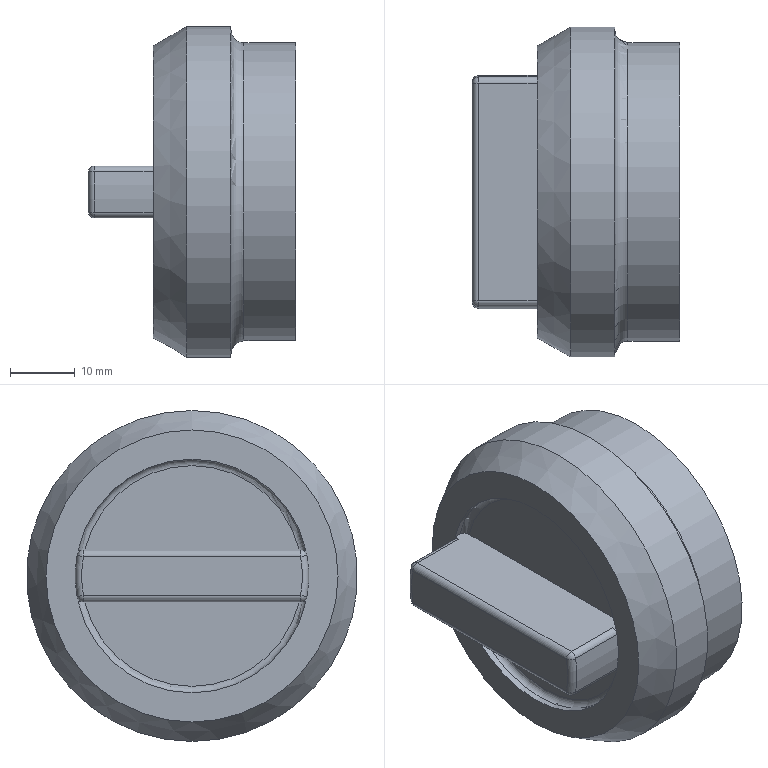Part | NX | features BLEND 3, DATUM_CSYS 3, SKETCH 2, CHAMFER 1, CYLINDER 1, EXTRUDE 1, HOLE PACKAGE 1, SIMPLE HOLE 1, SWP104 1, SYMBOLIC_THREAD 1 | 1 solid | 36 faces | box 32 x 51 x 51 mm | volume 28582 mm3 | cylinder 14 | plane 10 | torus 5 | sphere 4 | cone 3 | commonest cylinder face diameters 2 x6 36 x4 33 x1 36.5 x1 46 x1 51 x1
STEP:
#1=CARTESIAN_POINT('',(-21.,-17.55,4.));
#2=VERTEX_POINT('',#1);
#3=CARTESIAN_POINT('',(-22.,-17.55,4.));
#4=VERTEX_POINT('',#3);
#5=CARTESIAN_POINT('',(-32.,-17.55,4.));
#6=DIRECTION('',(1.,0.,0.));
#7=VECTOR('',#6,1000.);
#8=LINE('',#5,#7);
#9=EDGE_CURVE('',#2,#4,#8,.F.);
#10=ORIENTED_EDGE('',*,*,#9,.T.);
#11=CARTESIAN_POINT('',(-22.,17.55,4.));
#12=VERTEX_POINT('',#11);
#13=CARTESIAN_POINT('',(-22.,0.,0.));
#14=DIRECTION('',(-1.,0.,0.));
#15=DIRECTION('',(0.,0.,1.));
#16=AXIS2_PLACEMENT_3D('',#13,#14,#15);
#17=CIRCLE('',#16,18.);
#18=EDGE_CURVE('',#4,#12,#17,.T.);
#19=ORIENTED_EDGE('',*,*,#18,.T.);
#20=CARTESIAN_POINT('',(-21.,17.55,4.));
#21=VERTEX_POINT('',#20);
#22=CARTESIAN_POINT('',(-32.,17.55,4.));
#23=DIRECTION('',(1.,0.,0.));
#24=VECTOR('',#23,1000.);
#25=LINE('',#22,#24);
#26=EDGE_CURVE('',#12,#21,#25,.T.);
#27=ORIENTED_EDGE('',*,*,#26,.T.);
#28=CARTESIAN_POINT('',(-21.,0.,0.));
#29=DIRECTION('',(-1.,0.,0.));
#30=DIRECTION('',(0.,0.,1.));
#31=AXIS2_PLACEMENT_3D('',#28,#29,#30);
#32=CIRCLE('',#31,18.);
#33=EDGE_CURVE('',#2,#21,#32,.T.);
#34=ORIENTED_EDGE('',*,*,#33,.F.);
#35=EDGE_LOOP('',(#10,#19,#27,#34));
#36=FACE_BOUND('',#35,.T.);
#37=CARTESIAN_POINT('',(0.,0.,0.));
#38=DIRECTION('',(-1.,0.,0.));
#39=DIRECTION('',(0.,0.,1.));
#40=AXIS2_PLACEMENT_3D('',#37,#38,#39);
#41=CYLINDRICAL_SURFACE('',#40,18.);
#42=ADVANCED_FACE('',(#36),#41,.F.);
#43=CARTESIAN_POINT('',(-22.,17.55,-4.));
#44=VERTEX_POINT('',#43);
#45=CARTESIAN_POINT('',(-22.,-17.55,-4.));
#46=VERTEX_POINT('',#45);
#47=CARTESIAN_POINT('',(-22.,0.,0.));
#48=DIRECTION('',(-1.,0.,0.));
#49=DIRECTION('',(0.,0.,1.));
#50=AXIS2_PLACEMENT_3D('',#47,#48,#49);
#51=CIRCLE('',#50,18.);
#52=EDGE_CURVE('',#44,#46,#51,.T.);
#53=ORIENTED_EDGE('',*,*,#52,.T.);
#54=CARTESIAN_POINT('',(-21.,-17.55,-4.));
#55=VERTEX_POINT('',#54);
#56=CARTESIAN_POINT('',(-32.,-17.55,-4.));
#57=DIRECTION('',(1.,0.,0.));
#58=VECTOR('',#57,1000.);
#59=LINE('',#56,#58);
#60=EDGE_CURVE('',#46,#55,#59,.T.);
#61=ORIENTED_EDGE('',*,*,#60,.T.);
#62=CARTESIAN_POINT('',(-21.,17.55,-4.));
#63=VERTEX_POINT('',#62);
#64=CARTESIAN_POINT('',(-21.,0.,0.));
#65=DIRECTION('',(-1.,0.,0.));
#66=DIRECTION('',(0.,0.,1.));
#67=AXIS2_PLACEMENT_3D('',#64,#65,#66);
#68=CIRCLE('',#67,18.);
#69=EDGE_CURVE('',#63,#55,#68,.T.);
#70=ORIENTED_EDGE('',*,*,#69,.F.);
#71=CARTESIAN_POINT('',(-32.,17.55,-4.));
#72=DIRECTION('',(1.,0.,0.));
#73=VECTOR('',#72,1000.);
#74=LINE('',#71,#73);
#75=EDGE_CURVE('',#63,#44,#74,.F.);
#76=ORIENTED_EDGE('',*,*,#75,.T.);
#77=EDGE_LOOP('',(#53,#61,#70,#76));
#78=FACE_BOUND('',#77,.T.);
#79=CARTESIAN_POINT('',(0.,0.,0.));
#80=DIRECTION('',(-1.,0.,0.));
#81=DIRECTION('',(0.,0.,1.));
#82=AXIS2_PLACEMENT_3D('',#79,#80,#81);
#83=CYLINDRICAL_SURFACE('',#82,18.);
#84=ADVANCED_FACE('',(#78),#83,.F.);
#85=CARTESIAN_POINT('',(-20.,-16.523,4.));
#86=VERTEX_POINT('',#85);
#87=CARTESIAN_POINT('',(-21.,-17.55,4.));
#88=CARTESIAN_POINT('',(-20.472,-17.55,4.));
#89=CARTESIAN_POINT('',(-20.,-17.052,4.));
#90=CARTESIAN_POINT('',(-20.,-16.523,4.));
#91=B_SPLINE_CURVE_WITH_KNOTS('',3,(#87,#88,#89,#90),.UNSPECIFIED.,.F.,.F.,(4,4),(0.006013,0.007597),.UNSPECIFIED.);
#92=EDGE_CURVE('',#2,#86,#91,.T.);
#93=ORIENTED_EDGE('',*,*,#92,.F.);
#94=ORIENTED_EDGE('',*,*,#33,.T.);
#95=CARTESIAN_POINT('',(-20.,16.523,4.));
#96=VERTEX_POINT('',#95);
#97=CARTESIAN_POINT('',(-20.,16.523,4.));
#98=CARTESIAN_POINT('',(-20.,17.055,4.));
#99=CARTESIAN_POINT('',(-20.471,17.55,4.));
#100=CARTESIAN_POINT('',(-21.,17.55,4.));
#101=B_SPLINE_CURVE_WITH_KNOTS('',3,(#97,#98,#99,#100),.UNSPECIFIED.,.F.,.F.,(4,4),(0.001306,0.002891),.UNSPECIFIED.);
#102=EDGE_CURVE('',#96,#21,#101,.T.);
#103=ORIENTED_EDGE('',*,*,#102,.F.);
#104=CARTESIAN_POINT('',(-20.,0.,0.));
#105=DIRECTION('',(-1.,0.,0.));
#106=DIRECTION('',(0.,0.,1.));
#107=AXIS2_PLACEMENT_3D('',#104,#105,#106);
#108=CIRCLE('',#107,17.);
#109=EDGE_CURVE('',#86,#96,#108,.T.);
#110=ORIENTED_EDGE('',*,*,#109,.F.);
#111=EDGE_LOOP('',(#93,#94,#103,#110));
#112=FACE_BOUND('',#111,.T.);
#113=CARTESIAN_POINT('',(-21.,0.,0.));
#114=DIRECTION('',(-1.,0.,0.));
#115=DIRECTION('',(0.,0.,1.));
#116=AXIS2_PLACEMENT_3D('',#113,#114,#115);
#117=TOROIDAL_SURFACE('',#116,17.,1.);
#118=ADVANCED_FACE('',(#112),#117,.F.);
#119=CARTESIAN_POINT('',(-20.,-16.523,-4.));
#120=VERTEX_POINT('',#119);
#121=CARTESIAN_POINT('',(-20.,-16.523,-4.));
#122=CARTESIAN_POINT('',(-20.,-17.057,-4.));
#123=CARTESIAN_POINT('',(-20.464,-17.55,-4.));
#124=CARTESIAN_POINT('',(-21.,-17.55,-4.));
#125=B_SPLINE_CURVE_WITH_KNOTS('',3,(#121,#122,#123,#124),.UNSPECIFIED.,.F.,.F.,(4,4),(0.005091,0.006676),.UNSPECIFIED.);
#126=EDGE_CURVE('',#120,#55,#125,.T.);
#127=ORIENTED_EDGE('',*,*,#126,.F.);
#128=CARTESIAN_POINT('',(-20.,16.523,-4.));
#129=VERTEX_POINT('',#128);
#130=CARTESIAN_POINT('',(-20.,0.,0.));
#131=DIRECTION('',(-1.,0.,0.));
#132=DIRECTION('',(0.,0.,1.));
#133=AXIS2_PLACEMENT_3D('',#130,#131,#132);
#134=CIRCLE('',#133,17.);
#135=EDGE_CURVE('',#129,#120,#134,.T.);
#136=ORIENTED_EDGE('',*,*,#135,.F.);
#137=CARTESIAN_POINT('',(-21.,17.55,-4.));
#138=CARTESIAN_POINT('',(-20.468,17.55,-4.));
#139=CARTESIAN_POINT('',(-20.,17.056,-4.));
#140=CARTESIAN_POINT('',(-20.,16.523,-4.));
#141=B_SPLINE_CURVE_WITH_KNOTS('',3,(#137,#138,#139,#140),.UNSPECIFIED.,.F.,.F.,(4,4),(0.003455,0.00504),.UNSPECIFIED.);
#142=EDGE_CURVE('',#63,#129,#141,.T.);
#143=ORIENTED_EDGE('',*,*,#142,.F.);
#144=ORIENTED_EDGE('',*,*,#69,.T.);
#145=EDGE_LOOP('',(#127,#136,#143,#144));
#146=FACE_BOUND('',#145,.T.);
#147=CARTESIAN_POINT('',(-21.,0.,0.));
#148=DIRECTION('',(-1.,0.,0.));
#149=DIRECTION('',(0.,0.,1.));
#150=AXIS2_PLACEMENT_3D('',#147,#148,#149);
#151=TOROIDAL_SURFACE('',#150,17.,1.);
#152=ADVANCED_FACE('',(#146),#151,.F.);
#153=CARTESIAN_POINT('',(-20.,17.55,-4.));
#154=DIRECTION('',(0.,-1.,0.));
#155=VECTOR('',#154,1000.);
#156=LINE('',#153,#155);
#157=EDGE_CURVE('',#129,#120,#156,.T.);
#158=ORIENTED_EDGE('',*,*,#157,.F.);
#159=ORIENTED_EDGE('',*,*,#135,.T.);
#160=EDGE_LOOP('',(#158,#159));
#161=FACE_BOUND('',#160,.T.);
#162=CARTESIAN_POINT('',(-20.,0.,17.));
#163=DIRECTION('',(1.,0.,0.));
#164=DIRECTION('',(0.,0.,-1.));
#165=AXIS2_PLACEMENT_3D('',#162,#163,#164);
#166=PLANE('',#165);
#167=ADVANCED_FACE('',(#161),#166,.F.);
#168=CARTESIAN_POINT('',(-20.,-17.55,4.));
#169=DIRECTION('',(0.,1.,0.));
#170=VECTOR('',#169,1000.);
#171=LINE('',#168,#170);
#172=EDGE_CURVE('',#86,#96,#171,.T.);
#173=ORIENTED_EDGE('',*,*,#172,.F.);
#174=ORIENTED_EDGE('',*,*,#109,.T.);
#175=EDGE_LOOP('',(#173,#174));
#176=FACE_BOUND('',#175,.T.);
#177=CARTESIAN_POINT('',(-20.,0.,17.));
#178=DIRECTION('',(1.,0.,0.));
#179=DIRECTION('',(0.,0.,-1.));
#180=AXIS2_PLACEMENT_3D('',#177,#178,#179);
#181=PLANE('',#180);
#182=ADVANCED_FACE('',(#176),#181,.F.);
#183=CARTESIAN_POINT('',(-22.,17.718,3.176));
#184=VERTEX_POINT('',#183);
#185=CARTESIAN_POINT('',(-22.,17.718,-3.176));
#186=VERTEX_POINT('',#185);
#187=CARTESIAN_POINT('',(-22.,0.,0.));
#188=DIRECTION('',(-1.,0.,0.));
#189=DIRECTION('',(0.,0.,1.));
#190=AXIS2_PLACEMENT_3D('',#187,#188,#189);
#191=CIRCLE('',#190,18.);
#192=EDGE_CURVE('',#184,#186,#191,.T.);
#193=ORIENTED_EDGE('',*,*,#192,.F.);
#194=CARTESIAN_POINT('',(-22.,16.733,4.));
#195=VERTEX_POINT('',#194);
#196=CARTESIAN_POINT('',(-22.,16.733,3.));
#197=DIRECTION('',(1.,0.,0.));
#198=DIRECTION('',(0.,0.,-1.));
#199=AXIS2_PLACEMENT_3D('',#196,#197,#198);
#200=CIRCLE('',#199,1.);
#201=EDGE_CURVE('',#184,#195,#200,.T.);
#202=ORIENTED_EDGE('',*,*,#201,.T.);
#203=CARTESIAN_POINT('',(-22.,-17.55,4.));
#204=DIRECTION('',(0.,-1.,0.));
#205=VECTOR('',#204,1000.);
#206=LINE('',#203,#205);
#207=EDGE_CURVE('',#12,#195,#206,.T.);
#208=ORIENTED_EDGE('',*,*,#207,.F.);
#209=ORIENTED_EDGE('',*,*,#18,.F.);
#210=CARTESIAN_POINT('',(-22.,-16.733,4.));
#211=VERTEX_POINT('',#210);
#212=CARTESIAN_POINT('',(-22.,-17.55,4.));
#213=DIRECTION('',(0.,-1.,0.));
#214=VECTOR('',#213,1000.);
#215=LINE('',#212,#214);
#216=EDGE_CURVE('',#211,#4,#215,.T.);
#217=ORIENTED_EDGE('',*,*,#216,.F.);
#218=CARTESIAN_POINT('',(-22.,-17.718,3.176));
#219=VERTEX_POINT('',#218);
#220=CARTESIAN_POINT('',(-22.,-16.733,3.));
#221=DIRECTION('',(1.,0.,0.));
#222=DIRECTION('',(0.,0.,-1.));
#223=AXIS2_PLACEMENT_3D('',#220,#221,#222);
#224=CIRCLE('',#223,1.);
#225=EDGE_CURVE('',#211,#219,#224,.T.);
#226=ORIENTED_EDGE('',*,*,#225,.T.);
#227=CARTESIAN_POINT('',(-22.,-17.718,-3.176));
#228=VERTEX_POINT('',#227);
#229=CARTESIAN_POINT('',(-22.,0.,0.));
#230=DIRECTION('',(-1.,0.,0.));
#231=DIRECTION('',(0.,0.,1.));
#232=AXIS2_PLACEMENT_3D('',#229,#230,#231);
#233=CIRCLE('',#232,18.);
#234=EDGE_CURVE('',#228,#219,#233,.T.);
#235=ORIENTED_EDGE('',*,*,#234,.F.);
#236=CARTESIAN_POINT('',(-22.,-16.733,-4.));
#237=VERTEX_POINT('',#236);
#238=CARTESIAN_POINT('',(-22.,-16.733,-3.));
#239=DIRECTION('',(1.,0.,0.));
#240=DIRECTION('',(0.,0.,-1.));
#241=AXIS2_PLACEMENT_3D('',#238,#239,#240);
#242=CIRCLE('',#241,1.);
#243=EDGE_CURVE('',#228,#237,#242,.T.);
#244=ORIENTED_EDGE('',*,*,#243,.T.);
#245=CARTESIAN_POINT('',(-22.,17.55,-4.));
#246=DIRECTION('',(0.,1.,0.));
#247=VECTOR('',#246,1000.);
#248=LINE('',#245,#247);
#249=EDGE_CURVE('',#46,#237,#248,.T.);
#250=ORIENTED_EDGE('',*,*,#249,.F.);
#251=ORIENTED_EDGE('',*,*,#52,.F.);
#252=CARTESIAN_POINT('',(-22.,16.733,-4.));
#253=VERTEX_POINT('',#252);
#254=CARTESIAN_POINT('',(-22.,17.55,-4.));
#255=DIRECTION('',(0.,1.,0.));
#256=VECTOR('',#255,1000.);
#257=LINE('',#254,#256);
#258=EDGE_CURVE('',#253,#44,#257,.T.);
#259=ORIENTED_EDGE('',*,*,#258,.F.);
#260=CARTESIAN_POINT('',(-22.,16.733,-3.));
#261=DIRECTION('',(1.,0.,0.));
#262=DIRECTION('',(0.,0.,-1.));
#263=AXIS2_PLACEMENT_3D('',#260,#261,#262);
#264=CIRCLE('',#263,1.);
#265=EDGE_CURVE('',#253,#186,#264,.T.);
#266=ORIENTED_EDGE('',*,*,#265,.T.);
#267=EDGE_LOOP('',(#193,#202,#208,#209,#217,#226,#235,#244,#250,#251,#259,#266));
#268=FACE_BOUND('',#267,.T.);
#269=CARTESIAN_POINT('',(-22.,0.,22.5));
#270=VERTEX_POINT('',#269);
#271=CARTESIAN_POINT('',(-22.,0.,0.));
#272=DIRECTION('',(-1.,0.,0.));
#273=DIRECTION('',(0.,0.,1.));
#274=AXIS2_PLACEMENT_3D('',#271,#272,#273);
#275=CIRCLE('',#274,22.5);
#276=EDGE_CURVE('',#270,#270,#275,.T.);
#277=ORIENTED_EDGE('',*,*,#276,.T.);
#278=EDGE_LOOP('',(#277));
#279=FACE_BOUND('',#278,.T.);
#280=CARTESIAN_POINT('',(-22.,0.,22.5));
#281=DIRECTION('',(1.,0.,0.));
#282=DIRECTION('',(0.,0.,-1.));
#283=AXIS2_PLACEMENT_3D('',#280,#281,#282);
#284=PLANE('',#283);
#285=ADVANCED_FACE('',(#268,#279),#284,.F.);
#286=CARTESIAN_POINT('',(0.,0.,18.));
#287=VERTEX_POINT('',#286);
#288=CARTESIAN_POINT('',(0.,0.,0.));
#289=DIRECTION('',(-1.,0.,0.));
#290=DIRECTION('',(0.,0.,1.));
#291=AXIS2_PLACEMENT_3D('',#288,#289,#290);
#292=CIRCLE('',#291,18.);
#293=EDGE_CURVE('',#287,#287,#292,.T.);
#294=ORIENTED_EDGE('',*,*,#293,.T.);
#295=EDGE_LOOP('',(#294));
#296=FACE_BOUND('',#295,.T.);
#297=CARTESIAN_POINT('',(0.,0.,23.));
#298=VERTEX_POINT('',#297);
#299=CARTESIAN_POINT('',(0.,0.,0.));
#300=DIRECTION('',(-1.,0.,0.));
#301=DIRECTION('',(0.,0.,1.));
#302=AXIS2_PLACEMENT_3D('',#299,#300,#301);
#303=CIRCLE('',#302,23.);
#304=EDGE_CURVE('',#298,#298,#303,.T.);
#305=ORIENTED_EDGE('',*,*,#304,.F.);
#306=EDGE_LOOP('',(#305));
#307=FACE_BOUND('',#306,.T.);
#308=CARTESIAN_POINT('',(0.,0.,0.));
#309=DIRECTION('',(-1.,0.,0.));
#310=DIRECTION('',(0.,0.,1.));
#311=AXIS2_PLACEMENT_3D('',#308,#309,#310);
#312=PLANE('',#311);
#313=ADVANCED_FACE('',(#296,#307),#312,.F.);
#314=CARTESIAN_POINT('',(-8.,0.,23.));
#315=VERTEX_POINT('',#314);
#316=CARTESIAN_POINT('',(-8.,0.,0.));
#317=DIRECTION('',(-1.,0.,0.));
#318=DIRECTION('',(0.,0.,1.));
#319=AXIS2_PLACEMENT_3D('',#316,#317,#318);
#320=CIRCLE('',#319,23.);
#321=EDGE_CURVE('',#315,#315,#320,.T.);
#322=ORIENTED_EDGE('',*,*,#321,.F.);
#323=EDGE_LOOP('',(#322));
#324=FACE_BOUND('',#323,.T.);
#325=ORIENTED_EDGE('',*,*,#304,.T.);
#326=EDGE_LOOP('',(#325));
#327=FACE_BOUND('',#326,.T.);
#328=CARTESIAN_POINT('',(0.,0.,0.));
#329=DIRECTION('',(-1.,0.,0.));
#330=DIRECTION('',(0.,0.,1.));
#331=AXIS2_PLACEMENT_3D('',#328,#329,#330);
#332=CYLINDRICAL_SURFACE('',#331,23.);
#333=ADVANCED_FACE('',(#324,#327),#332,.T.);
#334=CARTESIAN_POINT('',(-10.,0.,25.));
#335=VERTEX_POINT('',#334);
#336=CARTESIAN_POINT('',(-10.,0.,0.));
#337=DIRECTION('',(-1.,0.,0.));
#338=DIRECTION('',(0.,0.,1.));
#339=AXIS2_PLACEMENT_3D('',#336,#337,#338);
#340=CIRCLE('',#339,25.);
#341=EDGE_CURVE('',#335,#335,#340,.T.);
#342=ORIENTED_EDGE('',*,*,#341,.F.);
#343=EDGE_LOOP('',(#342));
#344=FACE_BOUND('',#343,.T.);
#345=ORIENTED_EDGE('',*,*,#321,.T.);
#346=EDGE_LOOP('',(#345));
#347=FACE_BOUND('',#346,.T.);
#348=CARTESIAN_POINT('',(-8.,0.,0.));
#349=DIRECTION('',(-1.,0.,0.));
#350=DIRECTION('',(0.,0.,1.));
#351=AXIS2_PLACEMENT_3D('',#348,#349,#350);
#352=TOROIDAL_SURFACE('',#351,25.,2.);
#353=ADVANCED_FACE('',(#344,#347),#352,.F.);
#354=CARTESIAN_POINT('',(-10.,0.,25.5));
#355=VERTEX_POINT('',#354);
#356=CARTESIAN_POINT('',(-10.,0.,0.));
#357=DIRECTION('',(-1.,0.,0.));
#358=DIRECTION('',(0.,0.,1.));
#359=AXIS2_PLACEMENT_3D('',#356,#357,#358);
#360=CIRCLE('',#359,25.5);
#361=EDGE_CURVE('',#355,#355,#360,.T.);
#362=ORIENTED_EDGE('',*,*,#361,.F.);
#363=EDGE_LOOP('',(#362));
#364=FACE_BOUND('',#363,.T.);
#365=ORIENTED_EDGE('',*,*,#341,.T.);
#366=EDGE_LOOP('',(#365));
#367=FACE_BOUND('',#366,.T.);
#368=CARTESIAN_POINT('',(-10.,0.,25.));
#369=DIRECTION('',(-1.,0.,0.));
#370=DIRECTION('',(0.,0.,1.));
#371=AXIS2_PLACEMENT_3D('',#368,#369,#370);
#372=PLANE('',#371);
#373=ADVANCED_FACE('',(#364,#367),#372,.F.);
#374=CARTESIAN_POINT('',(-16.804,0.,25.5));
#375=VERTEX_POINT('',#374);
#376=CARTESIAN_POINT('',(-16.804,0.,0.));
#377=DIRECTION('',(-1.,0.,0.));
#378=DIRECTION('',(0.,0.,1.));
#379=AXIS2_PLACEMENT_3D('',#376,#377,#378);
#380=CIRCLE('',#379,25.5);
#381=EDGE_CURVE('',#375,#375,#380,.T.);
#382=ORIENTED_EDGE('',*,*,#381,.F.);
#383=EDGE_LOOP('',(#382));
#384=FACE_BOUND('',#383,.T.);
#385=ORIENTED_EDGE('',*,*,#361,.T.);
#386=EDGE_LOOP('',(#385));
#387=FACE_BOUND('',#386,.T.);
#388=CARTESIAN_POINT('',(0.,0.,0.));
#389=DIRECTION('',(-1.,0.,0.));
#390=DIRECTION('',(0.,0.,1.));
#391=AXIS2_PLACEMENT_3D('',#388,#389,#390);
#392=CYLINDRICAL_SURFACE('',#391,25.5);
#393=ADVANCED_FACE('',(#384,#387),#392,.T.);
#394=ORIENTED_EDGE('',*,*,#276,.F.);
#395=EDGE_LOOP('',(#394));
#396=FACE_BOUND('',#395,.T.);
#397=ORIENTED_EDGE('',*,*,#381,.T.);
#398=EDGE_LOOP('',(#397));
#399=FACE_BOUND('',#398,.T.);
#400=CARTESIAN_POINT('',(-16.804,0.,0.));
#401=DIRECTION('',(1.,0.,0.));
#402=DIRECTION('',(0.,0.,-1.));
#403=AXIS2_PLACEMENT_3D('',#400,#401,#402);
#404=CONICAL_SURFACE('',#403,25.5,0.5236);
#405=ADVANCED_FACE('',(#396,#399),#404,.T.);
#406=CARTESIAN_POINT('',(-2.,0.,-16.5));
#407=VERTEX_POINT('',#406);
#408=CARTESIAN_POINT('',(-2.,0.,0.));
#409=DIRECTION('',(1.,0.,0.));
#410=DIRECTION('',(0.,0.,-1.));
#411=AXIS2_PLACEMENT_3D('',#408,#409,#410);
#412=CIRCLE('',#411,16.5);
#413=EDGE_CURVE('',#407,#407,#412,.T.);
#414=ORIENTED_EDGE('',*,*,#413,.T.);
#415=EDGE_LOOP('',(#414));
#416=FACE_BOUND('',#415,.T.);
#417=CARTESIAN_POINT('',(-10.,0.,16.5));
#418=VERTEX_POINT('',#417);
#419=CARTESIAN_POINT('',(-10.,0.,0.));
#420=DIRECTION('',(-1.,0.,0.));
#421=DIRECTION('',(0.,0.,1.));
#422=AXIS2_PLACEMENT_3D('',#419,#420,#421);
#423=CIRCLE('',#422,16.5);
#424=EDGE_CURVE('',#418,#418,#423,.F.);
#425=ORIENTED_EDGE('',*,*,#424,.F.);
#426=EDGE_LOOP('',(#425));
#427=FACE_BOUND('',#426,.T.);
#428=CARTESIAN_POINT('',(0.,0.,0.));
#429=DIRECTION('',(-1.,0.,0.));
#430=DIRECTION('',(0.,0.,1.));
#431=AXIS2_PLACEMENT_3D('',#428,#429,#430);
#432=CYLINDRICAL_SURFACE('',#431,16.5);
#433=ADVANCED_FACE('',(#416,#427),#432,.F.);
#434=CARTESIAN_POINT('',(-1.146,0.,-16.854));
#435=VERTEX_POINT('',#434);
#436=CARTESIAN_POINT('',(-1.146,0.,0.));
#437=DIRECTION('',(1.,0.,0.));
#438=DIRECTION('',(0.,0.,-1.));
#439=AXIS2_PLACEMENT_3D('',#436,#437,#438);
#440=CIRCLE('',#439,16.854);
#441=EDGE_CURVE('',#435,#435,#440,.F.);
#442=ORIENTED_EDGE('',*,*,#441,.T.);
#443=EDGE_LOOP('',(#442));
#444=FACE_BOUND('',#443,.T.);
#445=ORIENTED_EDGE('',*,*,#293,.F.);
#446=EDGE_LOOP('',(#445));
#447=FACE_BOUND('',#446,.T.);
#448=CARTESIAN_POINT('',(0.,0.,0.));
#449=DIRECTION('',(1.,0.,0.));
#450=DIRECTION('',(0.,0.,-1.));
#451=AXIS2_PLACEMENT_3D('',#448,#449,#450);
#452=CONICAL_SURFACE('',#451,18.,0.7854);
#453=ADVANCED_FACE('',(#444,#447),#452,.F.);
#454=CARTESIAN_POINT('',(-14.,0.,18.25));
#455=VERTEX_POINT('',#454);
#456=CARTESIAN_POINT('',(-14.,0.,0.));
#457=DIRECTION('',(1.,0.,0.));
#458=DIRECTION('',(0.,0.,1.));
#459=AXIS2_PLACEMENT_3D('',#456,#457,#458);
#460=CIRCLE('',#459,18.25);
#461=EDGE_CURVE('',#455,#455,#460,.F.);
#462=ORIENTED_EDGE('',*,*,#461,.F.);
#463=EDGE_LOOP('',(#462));
#464=FACE_BOUND('',#463,.T.);
#465=CARTESIAN_POINT('',(-14.,0.,0.));
#466=DIRECTION('',(-1.,0.,0.));
#467=DIRECTION('',(0.,0.,1.));
#468=AXIS2_PLACEMENT_3D('',#465,#466,#467);
#469=PLANE('',#468);
#470=ADVANCED_FACE('',(#464),#469,.F.);
#471=ORIENTED_EDGE('',*,*,#424,.T.);
#472=EDGE_LOOP('',(#471));
#473=FACE_BOUND('',#472,.T.);
#474=CARTESIAN_POINT('',(-10.,0.,18.25));
#475=VERTEX_POINT('',#474);
#476=CARTESIAN_POINT('',(-10.,0.,0.));
#477=DIRECTION('',(-1.,0.,0.));
#478=DIRECTION('',(0.,0.,1.));
#479=AXIS2_PLACEMENT_3D('',#476,#477,#478);
#480=CIRCLE('',#479,18.25);
#481=EDGE_CURVE('',#475,#475,#480,.F.);
#482=ORIENTED_EDGE('',*,*,#481,.F.);
#483=EDGE_LOOP('',(#482));
#484=FACE_BOUND('',#483,.T.);
#485=CARTESIAN_POINT('',(-10.,0.,0.));
#486=DIRECTION('',(1.,0.,0.));
#487=DIRECTION('',(0.,0.,-1.));
#488=AXIS2_PLACEMENT_3D('',#485,#486,#487);
#489=PLANE('',#488);
#490=ADVANCED_FACE('',(#473,#484),#489,.F.);
#491=ORIENTED_EDGE('',*,*,#461,.T.);
#492=EDGE_LOOP('',(#491));
#493=FACE_BOUND('',#492,.T.);
#494=ORIENTED_EDGE('',*,*,#481,.T.);
#495=EDGE_LOOP('',(#494));
#496=FACE_BOUND('',#495,.T.);
#497=CARTESIAN_POINT('',(-10.,0.,0.));
#498=DIRECTION('',(-1.,0.,0.));
#499=DIRECTION('',(0.,0.,1.));
#500=AXIS2_PLACEMENT_3D('',#497,#498,#499);
#501=CYLINDRICAL_SURFACE('',#500,18.25);
#502=ADVANCED_FACE('',(#493,#496),#501,.F.);
#503=ORIENTED_EDGE('',*,*,#441,.F.);
#504=EDGE_LOOP('',(#503));
#505=FACE_BOUND('',#504,.T.);
#506=ORIENTED_EDGE('',*,*,#413,.F.);
#507=EDGE_LOOP('',(#506));
#508=FACE_BOUND('',#507,.T.);
#509=CARTESIAN_POINT('',(-2.,0.,0.));
#510=DIRECTION('',(1.,0.,0.));
#511=DIRECTION('',(0.,0.,-1.));
#512=AXIS2_PLACEMENT_3D('',#509,#510,#511);
#513=CONICAL_SURFACE('',#512,16.5,0.3927);
#514=ADVANCED_FACE('',(#505,#508),#513,.F.);
#515=CARTESIAN_POINT('',(-31.,-17.718,3.176));
#516=VERTEX_POINT('',#515);
#517=CARTESIAN_POINT('',(-31.,-17.718,-3.176));
#518=VERTEX_POINT('',#517);
#519=CARTESIAN_POINT('',(-31.,0.,0.));
#520=DIRECTION('',(-1.,0.,0.));
#521=DIRECTION('',(0.,0.,1.));
#522=AXIS2_PLACEMENT_3D('',#519,#520,#521);
#523=CIRCLE('',#522,18.);
#524=EDGE_CURVE('',#516,#518,#523,.F.);
#525=ORIENTED_EDGE('',*,*,#524,.T.);
#526=CARTESIAN_POINT('',(-32.,-17.718,-3.176));
#527=DIRECTION('',(1.,0.,0.));
#528=VECTOR('',#527,1000.);
#529=LINE('',#526,#528);
#530=EDGE_CURVE('',#518,#228,#529,.T.);
#531=ORIENTED_EDGE('',*,*,#530,.T.);
#532=ORIENTED_EDGE('',*,*,#234,.T.);
#533=CARTESIAN_POINT('',(-32.,-17.718,3.176));
#534=DIRECTION('',(1.,0.,0.));
#535=VECTOR('',#534,1000.);
#536=LINE('',#533,#535);
#537=EDGE_CURVE('',#219,#516,#536,.F.);
#538=ORIENTED_EDGE('',*,*,#537,.T.);
#539=EDGE_LOOP('',(#525,#531,#532,#538));
#540=FACE_BOUND('',#539,.T.);
#541=CARTESIAN_POINT('',(-32.,0.,0.));
#542=DIRECTION('',(1.,0.,0.));
#543=DIRECTION('',(0.,0.,-1.));
#544=AXIS2_PLACEMENT_3D('',#541,#542,#543);
#545=CYLINDRICAL_SURFACE('',#544,18.);
#546=ADVANCED_FACE('',(#540),#545,.T.);
#547=ORIENTED_EDGE('',*,*,#192,.T.);
#548=CARTESIAN_POINT('',(-31.,17.718,-3.176));
#549=VERTEX_POINT('',#548);
#550=CARTESIAN_POINT('',(-32.,17.718,-3.176));
#551=DIRECTION('',(1.,0.,0.));
#552=VECTOR('',#551,1000.);
#553=LINE('',#550,#552);
#554=EDGE_CURVE('',#186,#549,#553,.F.);
#555=ORIENTED_EDGE('',*,*,#554,.T.);
#556=CARTESIAN_POINT('',(-31.,17.718,3.176));
#557=VERTEX_POINT('',#556);
#558=CARTESIAN_POINT('',(-31.,0.,0.));
#559=DIRECTION('',(-1.,0.,0.));
#560=DIRECTION('',(0.,0.,1.));
#561=AXIS2_PLACEMENT_3D('',#558,#559,#560);
#562=CIRCLE('',#561,18.);
#563=EDGE_CURVE('',#549,#557,#562,.F.);
#564=ORIENTED_EDGE('',*,*,#563,.T.);
#565=CARTESIAN_POINT('',(-32.,17.718,3.176));
#566=DIRECTION('',(1.,0.,0.));
#567=VECTOR('',#566,1000.);
#568=LINE('',#565,#567);
#569=EDGE_CURVE('',#557,#184,#568,.T.);
#570=ORIENTED_EDGE('',*,*,#569,.T.);
#571=EDGE_LOOP('',(#547,#555,#564,#570));
#572=FACE_BOUND('',#571,.T.);
#573=CARTESIAN_POINT('',(-32.,0.,0.));
#574=DIRECTION('',(1.,0.,0.));
#575=DIRECTION('',(0.,0.,-1.));
#576=AXIS2_PLACEMENT_3D('',#573,#574,#575);
#577=CYLINDRICAL_SURFACE('',#576,18.);
#578=ADVANCED_FACE('',(#572),#577,.T.);
#579=ORIENTED_EDGE('',*,*,#26,.F.);
#580=ORIENTED_EDGE('',*,*,#207,.T.);
#581=CARTESIAN_POINT('',(-31.,16.733,4.));
#582=VERTEX_POINT('',#581);
#583=CARTESIAN_POINT('',(-32.,16.733,4.));
#584=DIRECTION('',(1.,0.,0.));
#585=VECTOR('',#584,1000.);
#586=LINE('',#583,#585);
#587=EDGE_CURVE('',#195,#582,#586,.F.);
#588=ORIENTED_EDGE('',*,*,#587,.T.);
#589=CARTESIAN_POINT('',(-31.,-16.733,4.));
#590=VERTEX_POINT('',#589);
#591=CARTESIAN_POINT('',(-31.,-17.55,4.));
#592=DIRECTION('',(0.,1.,0.));
#593=VECTOR('',#592,1000.);
#594=LINE('',#591,#593);
#595=EDGE_CURVE('',#582,#590,#594,.F.);
#596=ORIENTED_EDGE('',*,*,#595,.T.);
#597=CARTESIAN_POINT('',(-32.,-16.733,4.));
#598=DIRECTION('',(1.,0.,0.));
#599=VECTOR('',#598,1000.);
#600=LINE('',#597,#599);
#601=EDGE_CURVE('',#590,#211,#600,.T.);
#602=ORIENTED_EDGE('',*,*,#601,.T.);
#603=ORIENTED_EDGE('',*,*,#216,.T.);
#604=ORIENTED_EDGE('',*,*,#9,.F.);
#605=ORIENTED_EDGE('',*,*,#92,.T.);
#606=ORIENTED_EDGE('',*,*,#172,.T.);
#607=ORIENTED_EDGE('',*,*,#102,.T.);
#608=EDGE_LOOP('',(#579,#580,#588,#596,#602,#603,#604,#605,#606,#607));
#609=FACE_BOUND('',#608,.T.);
#610=CARTESIAN_POINT('',(-32.,-17.55,4.));
#611=DIRECTION('',(0.,0.,-1.));
#612=DIRECTION('',(-1.,0.,0.));
#613=AXIS2_PLACEMENT_3D('',#610,#611,#612);
#614=PLANE('',#613);
#615=ADVANCED_FACE('',(#609),#614,.F.);
#616=CARTESIAN_POINT('',(-31.,-16.733,-4.));
#617=VERTEX_POINT('',#616);
#618=CARTESIAN_POINT('',(-31.,16.733,-4.));
#619=VERTEX_POINT('',#618);
#620=CARTESIAN_POINT('',(-31.,17.55,-4.));
#621=DIRECTION('',(0.,-1.,0.));
#622=VECTOR('',#621,1000.);
#623=LINE('',#620,#622);
#624=EDGE_CURVE('',#617,#619,#623,.F.);
#625=ORIENTED_EDGE('',*,*,#624,.T.);
#626=CARTESIAN_POINT('',(-32.,16.733,-4.));
#627=DIRECTION('',(1.,0.,0.));
#628=VECTOR('',#627,1000.);
#629=LINE('',#626,#628);
#630=EDGE_CURVE('',#619,#253,#629,.T.);
#631=ORIENTED_EDGE('',*,*,#630,.T.);
#632=ORIENTED_EDGE('',*,*,#258,.T.);
#633=ORIENTED_EDGE('',*,*,#75,.F.);
#634=ORIENTED_EDGE('',*,*,#142,.T.);
#635=ORIENTED_EDGE('',*,*,#157,.T.);
#636=ORIENTED_EDGE('',*,*,#126,.T.);
#637=ORIENTED_EDGE('',*,*,#60,.F.);
#638=ORIENTED_EDGE('',*,*,#249,.T.);
#639=CARTESIAN_POINT('',(-32.,-16.733,-4.));
#640=DIRECTION('',(1.,0.,0.));
#641=VECTOR('',#640,1000.);
#642=LINE('',#639,#641);
#643=EDGE_CURVE('',#237,#617,#642,.F.);
#644=ORIENTED_EDGE('',*,*,#643,.T.);
#645=EDGE_LOOP('',(#625,#631,#632,#633,#634,#635,#636,#637,#638,#644));
#646=FACE_BOUND('',#645,.T.);
#647=CARTESIAN_POINT('',(-32.,17.55,-4.));
#648=DIRECTION('',(0.,0.,1.));
#649=DIRECTION('',(1.,0.,0.));
#650=AXIS2_PLACEMENT_3D('',#647,#648,#649);
#651=PLANE('',#650);
#652=ADVANCED_FACE('',(#646),#651,.F.);
#653=CARTESIAN_POINT('',(-32.,-16.733,3.));
#654=VERTEX_POINT('',#653);
#655=CARTESIAN_POINT('',(-32.,16.733,3.));
#656=VERTEX_POINT('',#655);
#657=CARTESIAN_POINT('',(-32.,17.55,3.));
#658=DIRECTION('',(0.,1.,0.));
#659=VECTOR('',#658,1000.);
#660=LINE('',#657,#659);
#661=EDGE_CURVE('',#654,#656,#660,.T.);
#662=ORIENTED_EDGE('',*,*,#661,.T.);
#663=CARTESIAN_POINT('',(-32.,16.733,-3.));
#664=VERTEX_POINT('',#663);
#665=CARTESIAN_POINT('',(-32.,0.,0.));
#666=DIRECTION('',(-1.,0.,0.));
#667=DIRECTION('',(0.,0.,1.));
#668=AXIS2_PLACEMENT_3D('',#665,#666,#667);
#669=CIRCLE('',#668,17.);
#670=EDGE_CURVE('',#656,#664,#669,.T.);
#671=ORIENTED_EDGE('',*,*,#670,.T.);
#672=CARTESIAN_POINT('',(-32.,-16.733,-3.));
#673=VERTEX_POINT('',#672);
#674=CARTESIAN_POINT('',(-32.,-17.55,-3.));
#675=DIRECTION('',(0.,-1.,0.));
#676=VECTOR('',#675,1000.);
#677=LINE('',#674,#676);
#678=EDGE_CURVE('',#664,#673,#677,.T.);
#679=ORIENTED_EDGE('',*,*,#678,.T.);
#680=CARTESIAN_POINT('',(-32.,0.,0.));
#681=DIRECTION('',(-1.,0.,0.));
#682=DIRECTION('',(0.,0.,1.));
#683=AXIS2_PLACEMENT_3D('',#680,#681,#682);
#684=CIRCLE('',#683,17.);
#685=EDGE_CURVE('',#673,#654,#684,.T.);
#686=ORIENTED_EDGE('',*,*,#685,.T.);
#687=EDGE_LOOP('',(#662,#671,#679,#686));
#688=FACE_BOUND('',#687,.T.);
#689=CARTESIAN_POINT('',(-32.,0.,0.));
#690=DIRECTION('',(-1.,0.,0.));
#691=DIRECTION('',(0.,0.,1.));
#692=AXIS2_PLACEMENT_3D('',#689,#690,#691);
#693=PLANE('',#692);
#694=ADVANCED_FACE('',(#688),#693,.T.);
#695=ORIENTED_EDGE('',*,*,#678,.F.);
#696=CARTESIAN_POINT('',(-31.,16.733,-3.));
#697=DIRECTION('',(0.,1.,0.));
#698=DIRECTION('',(0.,0.,1.));
#699=AXIS2_PLACEMENT_3D('',#696,#697,#698);
#700=CIRCLE('',#699,1.);
#701=EDGE_CURVE('',#664,#619,#700,.F.);
#702=ORIENTED_EDGE('',*,*,#701,.T.);
#703=ORIENTED_EDGE('',*,*,#624,.F.);
#704=CARTESIAN_POINT('',(-31.,-16.733,-3.));
#705=DIRECTION('',(0.,1.,0.));
#706=DIRECTION('',(0.,0.,1.));
#707=AXIS2_PLACEMENT_3D('',#704,#705,#706);
#708=CIRCLE('',#707,1.);
#709=EDGE_CURVE('',#617,#673,#708,.T.);
#710=ORIENTED_EDGE('',*,*,#709,.T.);
#711=EDGE_LOOP('',(#695,#702,#703,#710));
#712=FACE_BOUND('',#711,.T.);
#713=CARTESIAN_POINT('',(-31.,0.,-3.));
#714=DIRECTION('',(0.,1.,0.));
#715=DIRECTION('',(0.,0.,1.));
#716=AXIS2_PLACEMENT_3D('',#713,#714,#715);
#717=CYLINDRICAL_SURFACE('',#716,1.);
#718=ADVANCED_FACE('',(#712),#717,.T.);
#719=ORIENTED_EDGE('',*,*,#595,.F.);
#720=CARTESIAN_POINT('',(-31.,16.733,3.));
#721=DIRECTION('',(0.,-1.,0.));
#722=DIRECTION('',(0.,0.,-1.));
#723=AXIS2_PLACEMENT_3D('',#720,#721,#722);
#724=CIRCLE('',#723,1.);
#725=EDGE_CURVE('',#582,#656,#724,.T.);
#726=ORIENTED_EDGE('',*,*,#725,.T.);
#727=ORIENTED_EDGE('',*,*,#661,.F.);
#728=CARTESIAN_POINT('',(-31.,-16.733,3.));
#729=DIRECTION('',(0.,-1.,0.));
#730=DIRECTION('',(0.,0.,-1.));
#731=AXIS2_PLACEMENT_3D('',#728,#729,#730);
#732=CIRCLE('',#731,1.);
#733=EDGE_CURVE('',#654,#590,#732,.F.);
#734=ORIENTED_EDGE('',*,*,#733,.T.);
#735=EDGE_LOOP('',(#719,#726,#727,#734));
#736=FACE_BOUND('',#735,.T.);
#737=CARTESIAN_POINT('',(-31.,0.,3.));
#738=DIRECTION('',(0.,-1.,0.));
#739=DIRECTION('',(0.,0.,-1.));
#740=AXIS2_PLACEMENT_3D('',#737,#738,#739);
#741=CYLINDRICAL_SURFACE('',#740,1.);
#742=ADVANCED_FACE('',(#736),#741,.T.);
#743=ORIENTED_EDGE('',*,*,#225,.F.);
#744=ORIENTED_EDGE('',*,*,#601,.F.);
#745=CARTESIAN_POINT('',(-31.,-16.733,3.));
#746=DIRECTION('',(-1.,0.,0.));
#747=DIRECTION('',(0.,0.,1.));
#748=AXIS2_PLACEMENT_3D('',#745,#746,#747);
#749=CIRCLE('',#748,1.);
#750=EDGE_CURVE('',#516,#590,#749,.T.);
#751=ORIENTED_EDGE('',*,*,#750,.F.);
#752=ORIENTED_EDGE('',*,*,#537,.F.);
#753=EDGE_LOOP('',(#743,#744,#751,#752));
#754=FACE_BOUND('',#753,.T.);
#755=CARTESIAN_POINT('',(-32.,-16.733,3.));
#756=DIRECTION('',(1.,0.,0.));
#757=DIRECTION('',(0.,0.,-1.));
#758=AXIS2_PLACEMENT_3D('',#755,#756,#757);
#759=CYLINDRICAL_SURFACE('',#758,1.);
#760=ADVANCED_FACE('',(#754),#759,.T.);
#761=ORIENTED_EDGE('',*,*,#750,.T.);
#762=ORIENTED_EDGE('',*,*,#733,.F.);
#763=CARTESIAN_POINT('',(-31.,-16.733,3.));
#764=DIRECTION('',(0.,-0.1765,-0.9843));
#765=DIRECTION('',(0.,0.9843,-0.1765));
#766=AXIS2_PLACEMENT_3D('',#763,#764,#765);
#767=CIRCLE('',#766,1.);
#768=EDGE_CURVE('',#516,#654,#767,.T.);
#769=ORIENTED_EDGE('',*,*,#768,.F.);
#770=EDGE_LOOP('',(#761,#762,#769));
#771=FACE_BOUND('',#770,.T.);
#772=CARTESIAN_POINT('',(-31.,-16.733,3.));
#773=DIRECTION('',(0.,0.9843,-0.1765));
#774=DIRECTION('',(0.,0.1765,0.9843));
#775=AXIS2_PLACEMENT_3D('',#772,#773,#774);
#776=SPHERICAL_SURFACE('',#775,1.);
#777=ADVANCED_FACE('',(#771),#776,.T.);
#778=ORIENTED_EDGE('',*,*,#768,.T.);
#779=ORIENTED_EDGE('',*,*,#685,.F.);
#780=CARTESIAN_POINT('',(-31.,-16.733,-3.));
#781=DIRECTION('',(0.,0.1765,-0.9843));
#782=DIRECTION('',(0.,0.9843,0.1765));
#783=AXIS2_PLACEMENT_3D('',#780,#781,#782);
#784=CIRCLE('',#783,1.);
#785=EDGE_CURVE('',#518,#673,#784,.T.);
#786=ORIENTED_EDGE('',*,*,#785,.F.);
#787=ORIENTED_EDGE('',*,*,#524,.F.);
#788=EDGE_LOOP('',(#778,#779,#786,#787));
#789=FACE_BOUND('',#788,.T.);
#790=CARTESIAN_POINT('',(-31.,0.,0.));
#791=DIRECTION('',(-1.,0.,0.));
#792=DIRECTION('',(0.,0.,1.));
#793=AXIS2_PLACEMENT_3D('',#790,#791,#792);
#794=TOROIDAL_SURFACE('',#793,17.,1.);
#795=ADVANCED_FACE('',(#789),#794,.T.);
#796=ORIENTED_EDGE('',*,*,#785,.T.);
#797=ORIENTED_EDGE('',*,*,#709,.F.);
#798=CARTESIAN_POINT('',(-31.,-16.733,-3.));
#799=DIRECTION('',(1.,0.,0.));
#800=DIRECTION('',(0.,0.,-1.));
#801=AXIS2_PLACEMENT_3D('',#798,#799,#800);
#802=CIRCLE('',#801,1.);
#803=EDGE_CURVE('',#518,#617,#802,.T.);
#804=ORIENTED_EDGE('',*,*,#803,.F.);
#805=EDGE_LOOP('',(#796,#797,#804));
#806=FACE_BOUND('',#805,.T.);
#807=CARTESIAN_POINT('',(-31.,-16.733,-3.));
#808=DIRECTION('',(0.,0.9843,0.1765));
#809=DIRECTION('',(0.,-0.1765,0.9843));
#810=AXIS2_PLACEMENT_3D('',#807,#808,#809);
#811=SPHERICAL_SURFACE('',#810,1.);
#812=ADVANCED_FACE('',(#806),#811,.T.);
#813=ORIENTED_EDGE('',*,*,#803,.T.);
#814=ORIENTED_EDGE('',*,*,#643,.F.);
#815=ORIENTED_EDGE('',*,*,#243,.F.);
#816=ORIENTED_EDGE('',*,*,#530,.F.);
#817=EDGE_LOOP('',(#813,#814,#815,#816));
#818=FACE_BOUND('',#817,.T.);
#819=CARTESIAN_POINT('',(-32.,-16.733,-3.));
#820=DIRECTION('',(1.,0.,0.));
#821=DIRECTION('',(0.,0.,-1.));
#822=AXIS2_PLACEMENT_3D('',#819,#820,#821);
#823=CYLINDRICAL_SURFACE('',#822,1.);
#824=ADVANCED_FACE('',(#818),#823,.T.);
#825=CARTESIAN_POINT('',(-31.,16.733,3.));
#826=DIRECTION('',(-1.,0.,0.));
#827=DIRECTION('',(0.,0.,1.));
#828=AXIS2_PLACEMENT_3D('',#825,#826,#827);
#829=CIRCLE('',#828,1.);
#830=EDGE_CURVE('',#582,#557,#829,.T.);
#831=ORIENTED_EDGE('',*,*,#830,.F.);
#832=ORIENTED_EDGE('',*,*,#587,.F.);
#833=ORIENTED_EDGE('',*,*,#201,.F.);
#834=ORIENTED_EDGE('',*,*,#569,.F.);
#835=EDGE_LOOP('',(#831,#832,#833,#834));
#836=FACE_BOUND('',#835,.T.);
#837=CARTESIAN_POINT('',(-32.,16.733,3.));
#838=DIRECTION('',(1.,0.,0.));
#839=DIRECTION('',(0.,0.,-1.));
#840=AXIS2_PLACEMENT_3D('',#837,#838,#839);
#841=CYLINDRICAL_SURFACE('',#840,1.);
#842=ADVANCED_FACE('',(#836),#841,.T.);
#843=ORIENTED_EDGE('',*,*,#725,.F.);
#844=ORIENTED_EDGE('',*,*,#830,.T.);
#845=CARTESIAN_POINT('',(-31.,16.733,3.));
#846=DIRECTION('',(0.,0.1765,-0.9843));
#847=DIRECTION('',(0.,0.9843,0.1765));
#848=AXIS2_PLACEMENT_3D('',#845,#846,#847);
#849=CIRCLE('',#848,1.);
#850=EDGE_CURVE('',#656,#557,#849,.T.);
#851=ORIENTED_EDGE('',*,*,#850,.F.);
#852=EDGE_LOOP('',(#843,#844,#851));
#853=FACE_BOUND('',#852,.T.);
#854=CARTESIAN_POINT('',(-31.,16.733,3.));
#855=DIRECTION('',(0.,-0.9843,-0.1765));
#856=DIRECTION('',(0.,0.1765,-0.9843));
#857=AXIS2_PLACEMENT_3D('',#854,#855,#856);
#858=SPHERICAL_SURFACE('',#857,1.);
#859=ADVANCED_FACE('',(#853),#858,.T.);
#860=CARTESIAN_POINT('',(-31.,16.733,-3.));
#861=DIRECTION('',(0.,-0.1765,-0.9843));
#862=DIRECTION('',(0.,0.9843,-0.1765));
#863=AXIS2_PLACEMENT_3D('',#860,#861,#862);
#864=CIRCLE('',#863,1.);
#865=EDGE_CURVE('',#664,#549,#864,.T.);
#866=ORIENTED_EDGE('',*,*,#865,.F.);
#867=ORIENTED_EDGE('',*,*,#670,.F.);
#868=ORIENTED_EDGE('',*,*,#850,.T.);
#869=ORIENTED_EDGE('',*,*,#563,.F.);
#870=EDGE_LOOP('',(#866,#867,#868,#869));
#871=FACE_BOUND('',#870,.T.);
#872=CARTESIAN_POINT('',(-31.,0.,0.));
#873=DIRECTION('',(-1.,0.,0.));
#874=DIRECTION('',(0.,0.,1.));
#875=AXIS2_PLACEMENT_3D('',#872,#873,#874);
#876=TOROIDAL_SURFACE('',#875,17.,1.);
#877=ADVANCED_FACE('',(#871),#876,.T.);
#878=ORIENTED_EDGE('',*,*,#701,.F.);
#879=ORIENTED_EDGE('',*,*,#865,.T.);
#880=CARTESIAN_POINT('',(-31.,16.733,-3.));
#881=DIRECTION('',(1.,0.,0.));
#882=DIRECTION('',(0.,0.,-1.));
#883=AXIS2_PLACEMENT_3D('',#880,#881,#882);
#884=CIRCLE('',#883,1.);
#885=EDGE_CURVE('',#619,#549,#884,.T.);
#886=ORIENTED_EDGE('',*,*,#885,.F.);
#887=EDGE_LOOP('',(#878,#879,#886));
#888=FACE_BOUND('',#887,.T.);
#889=CARTESIAN_POINT('',(-31.,16.733,-3.));
#890=DIRECTION('',(0.,-0.9843,0.1765));
#891=DIRECTION('',(0.,-0.1765,-0.9843));
#892=AXIS2_PLACEMENT_3D('',#889,#890,#891);
#893=SPHERICAL_SURFACE('',#892,1.);
#894=ADVANCED_FACE('',(#888),#893,.T.);
#895=ORIENTED_EDGE('',*,*,#885,.T.);
#896=ORIENTED_EDGE('',*,*,#554,.F.);
#897=ORIENTED_EDGE('',*,*,#265,.F.);
#898=ORIENTED_EDGE('',*,*,#630,.F.);
#899=EDGE_LOOP('',(#895,#896,#897,#898));
#900=FACE_BOUND('',#899,.T.);
#901=CARTESIAN_POINT('',(-32.,16.733,-3.));
#902=DIRECTION('',(1.,0.,0.));
#903=DIRECTION('',(0.,0.,-1.));
#904=AXIS2_PLACEMENT_3D('',#901,#902,#903);
#905=CYLINDRICAL_SURFACE('',#904,1.);
#906=ADVANCED_FACE('',(#900),#905,.T.);
#907=CLOSED_SHELL('',(#42,#84,#118,#152,#167,#182,#285,#313,#333,#353,#373,#393,#405,#433,#453,#470,#490,#502,#514,#546,#578,#615,#652,#694,#718,#742,#760,#777,#795,#812,#824,#842,#859,#877,#894,#906));
#908=MANIFOLD_SOLID_BREP('',#907);
#909=(LENGTH_UNIT()NAMED_UNIT(*)SI_UNIT(.MILLI.,.METRE.));
#910=UNCERTAINTY_MEASURE_WITH_UNIT(LENGTH_MEASURE(0.0508),#909,'','');
#911=(NAMED_UNIT(*)PLANE_ANGLE_UNIT()SI_UNIT($,.RADIAN.));
#912=(NAMED_UNIT(*)SI_UNIT($,.STERADIAN.)SOLID_ANGLE_UNIT());
#913=(GEOMETRIC_REPRESENTATION_CONTEXT(3)GLOBAL_UNCERTAINTY_ASSIGNED_CONTEXT((#910))GLOBAL_UNIT_ASSIGNED_CONTEXT((#909,#911,#912))REPRESENTATION_CONTEXT('',''));
#914=ADVANCED_BREP_SHAPE_REPRESENTATION('',(#908),#913);